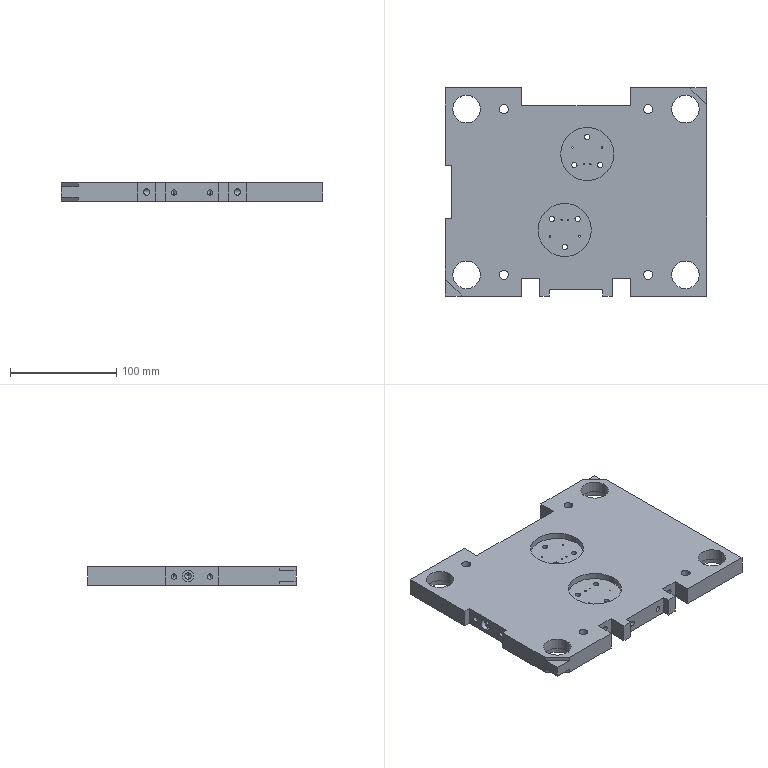Part | STEP file | 3 | 1 solid | 148 faces | box 246 x 196 x 17 mm | volume 676741 mm3 | cylinder 86 | plane 42 | cone 20 | commonest cylinder face diameters 5 x20 6 x18 1.4 x16 8.376 x8 26 x8 32 x8